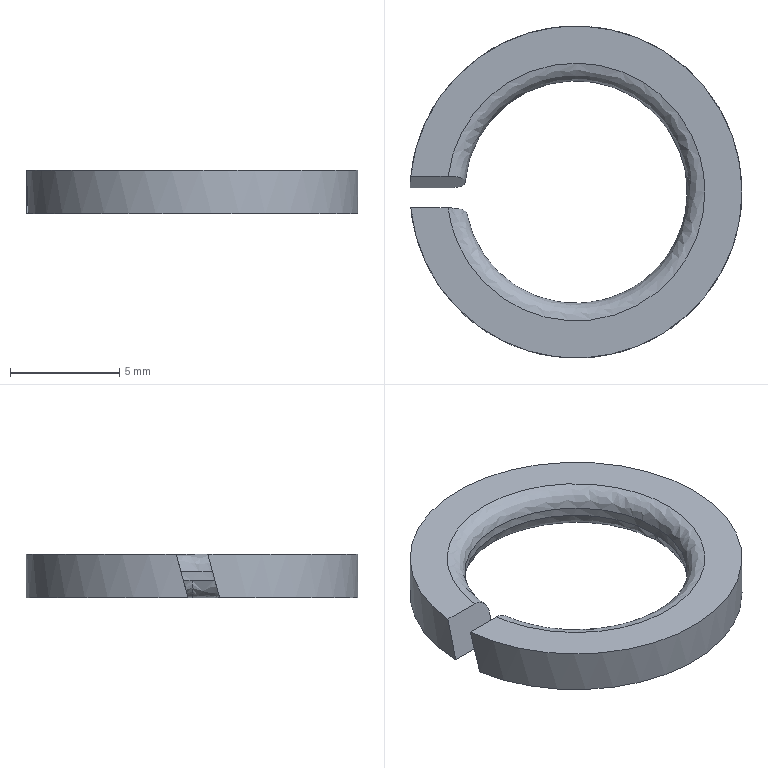Part | STEP file | 44 | 1 solid | 9 faces | box 15.198 x 15.2 x 2 mm | volume 183.52 mm3 | plane 4 | spline 3 | cylinder 2 | commonest cylinder face diameters 10.2 x1 15.2 x1